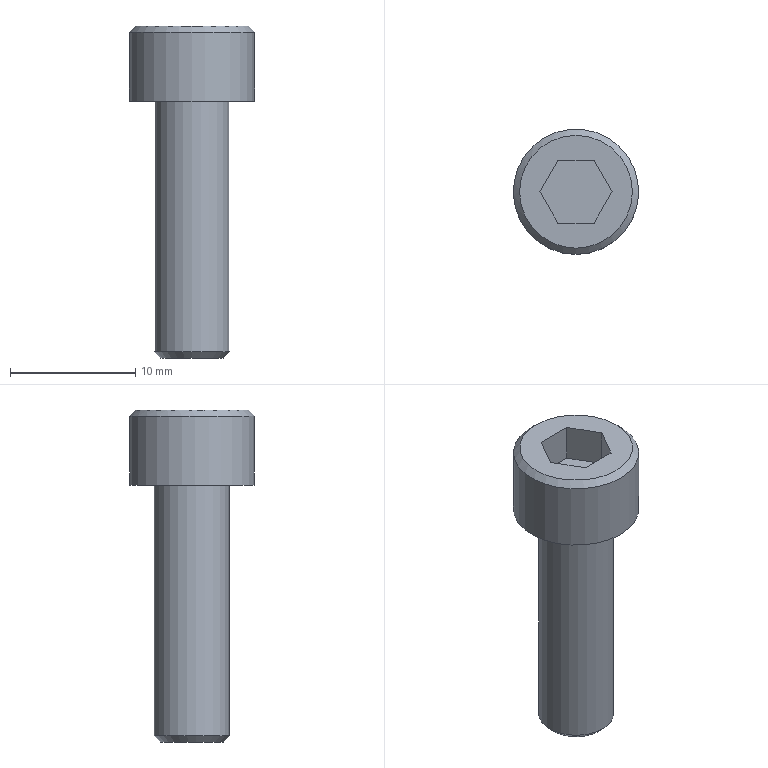Part | STEP file | solid 128 | 1 solid | 14 faces | box 10 x 10 x 26.5 mm | volume 979.889 mm3 | plane 10 | cone 2 | cylinder 2 | commonest cylinder face diameters 6 x1 10 x1